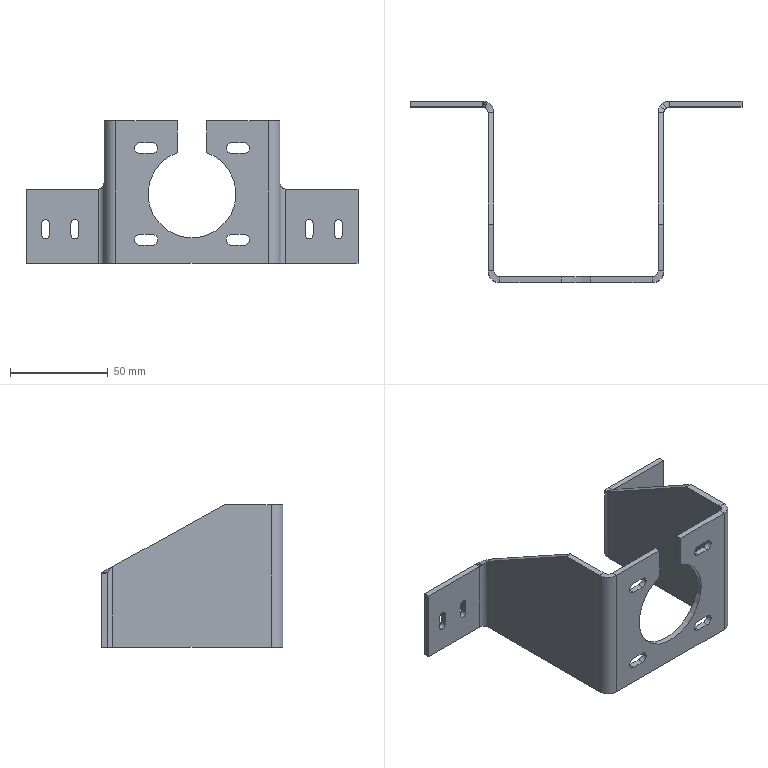Part | STEP file | Lift screen drive 57 mounting plate 001 | 1 solid | 82 faces | box 170 x 93 x 73 mm | volume 53723 mm3 | plane 49 | cylinder 25 | spline 8 | commonest cylinder face diameters 4 x8 5.5 x8 6 x4 12 x4 45 x1